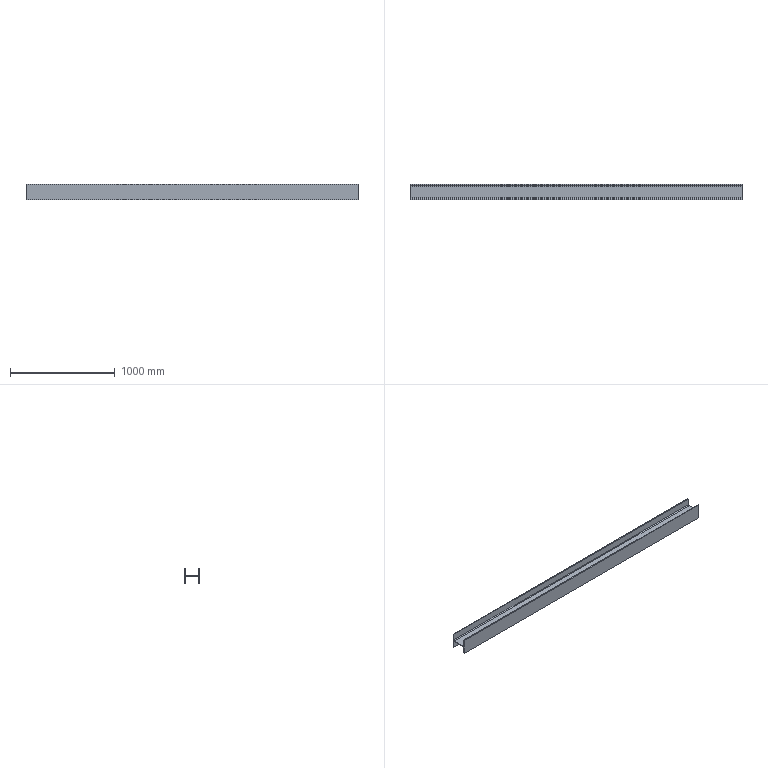Part | STEP file | 01-Cross beam H150X150_default<machining> | 1 solid | 22 faces | box 3170 x 150 x 150 mm | volume 12529220 mm3 | plane 16 | cylinder 6 | commonest cylinder face diameters 16 x4 100 x2